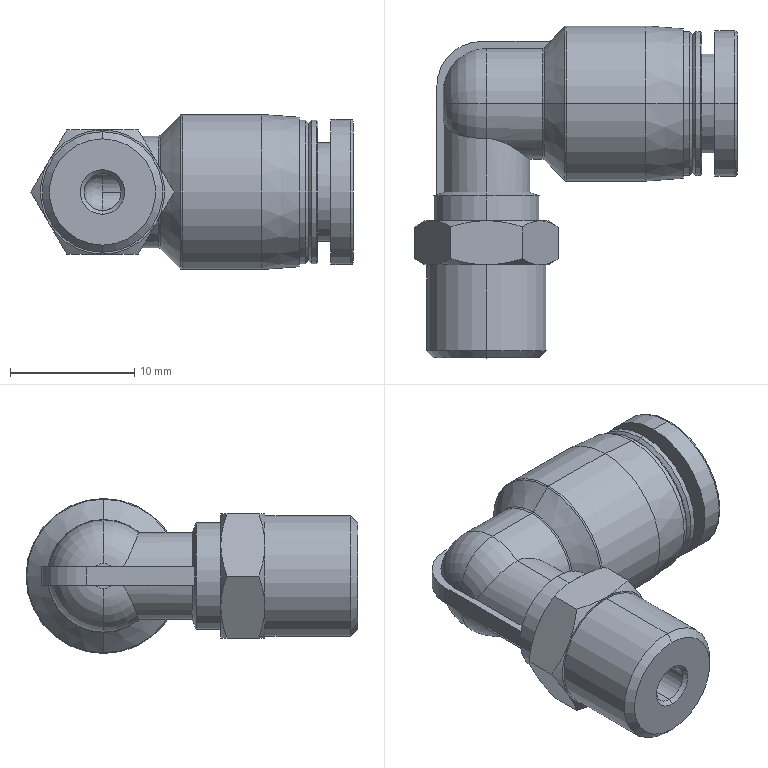Part | STEP file | PL601_HI | 1 solid | 93 faces | box 25.974 x 26.75 x 12.5 mm | volume 2654 mm3 | cone 28 | cylinder 27 | plane 20 | torus 13 | other 4 | sphere 1 | commonest cylinder face diameters 3 x4 11.6 x4 7 x3 9 x3 6 x2 8 x2